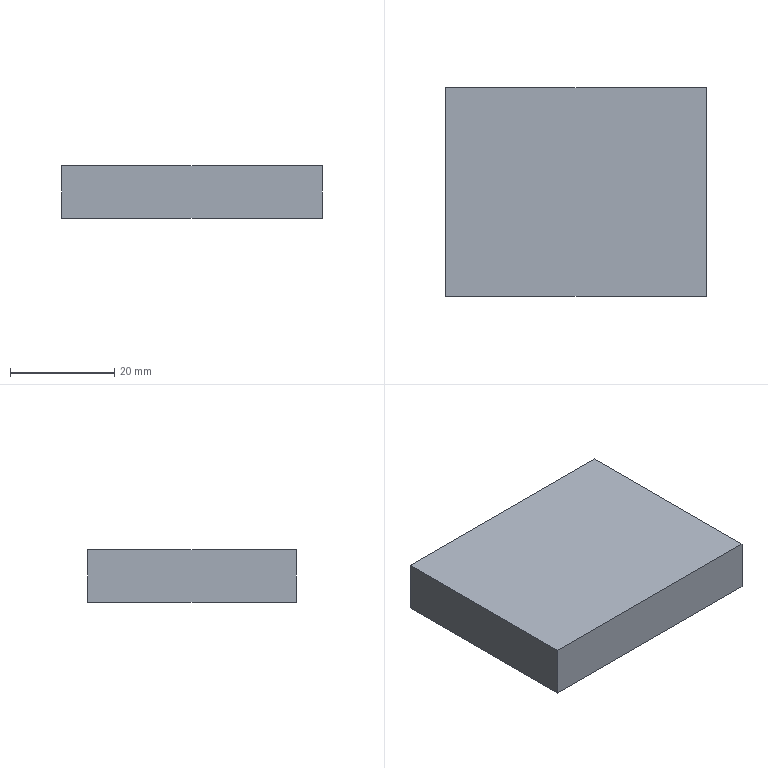Part | NX | features solid 2 | 1 solid | 6 faces | box 50 x 40 x 10 mm | volume 20000 mm3 | plane 6
STEP:
#1=CARTESIAN_POINT('',(604.,205.,-35.));
#2=VERTEX_POINT('',#1);
#3=CARTESIAN_POINT('',(604.,165.,-35.));
#4=VERTEX_POINT('',#3);
#5=CARTESIAN_POINT('',(604.,184.697,-35.));
#6=DIRECTION('',(0.,-1.,0.));
#7=VECTOR('',#6,1000.);
#8=LINE('',#5,#7);
#9=EDGE_CURVE('',#2,#4,#8,.T.);
#10=ORIENTED_EDGE('',*,*,#9,.F.);
#11=CARTESIAN_POINT('',(604.,205.,-45.));
#12=VERTEX_POINT('',#11);
#13=CARTESIAN_POINT('',(604.,205.,-45.));
#14=DIRECTION('',(0.,0.,1.));
#15=VECTOR('',#14,1000.);
#16=LINE('',#13,#15);
#17=EDGE_CURVE('',#12,#2,#16,.T.);
#18=ORIENTED_EDGE('',*,*,#17,.F.);
#19=CARTESIAN_POINT('',(604.,165.,-45.));
#20=VERTEX_POINT('',#19);
#21=CARTESIAN_POINT('',(604.,205.,-45.));
#22=DIRECTION('',(0.,1.,0.));
#23=VECTOR('',#22,1000.);
#24=LINE('',#21,#23);
#25=EDGE_CURVE('',#12,#20,#24,.F.);
#26=ORIENTED_EDGE('',*,*,#25,.T.);
#27=CARTESIAN_POINT('',(604.,165.,-50.));
#28=DIRECTION('',(0.,0.,1.));
#29=VECTOR('',#28,1000.);
#30=LINE('',#27,#29);
#31=EDGE_CURVE('',#20,#4,#30,.T.);
#32=ORIENTED_EDGE('',*,*,#31,.T.);
#33=EDGE_LOOP('',(#10,#18,#26,#32));
#34=FACE_BOUND('',#33,.T.);
#35=CARTESIAN_POINT('',(604.,205.,-45.));
#36=DIRECTION('',(1.,0.,0.));
#37=DIRECTION('',(0.,0.,-1.));
#38=AXIS2_PLACEMENT_3D('',#35,#36,#37);
#39=PLANE('',#38);
#40=ADVANCED_FACE('',(#34),#39,.F.);
#41=CARTESIAN_POINT('',(654.,205.,-35.));
#42=VERTEX_POINT('',#41);
#43=CARTESIAN_POINT('',(654.,165.,-35.));
#44=VERTEX_POINT('',#43);
#45=CARTESIAN_POINT('',(654.,184.697,-35.));
#46=DIRECTION('',(0.,1.,0.));
#47=VECTOR('',#46,1000.);
#48=LINE('',#45,#47);
#49=EDGE_CURVE('',#42,#44,#48,.F.);
#50=ORIENTED_EDGE('',*,*,#49,.T.);
#51=CARTESIAN_POINT('',(654.,165.,-45.));
#52=VERTEX_POINT('',#51);
#53=CARTESIAN_POINT('',(654.,165.,-50.));
#54=DIRECTION('',(0.,0.,-1.));
#55=VECTOR('',#54,1000.);
#56=LINE('',#53,#55);
#57=EDGE_CURVE('',#52,#44,#56,.F.);
#58=ORIENTED_EDGE('',*,*,#57,.F.);
#59=CARTESIAN_POINT('',(654.,205.,-45.));
#60=VERTEX_POINT('',#59);
#61=CARTESIAN_POINT('',(654.,205.,-45.));
#62=DIRECTION('',(0.,-1.,0.));
#63=VECTOR('',#62,1000.);
#64=LINE('',#61,#63);
#65=EDGE_CURVE('',#60,#52,#64,.T.);
#66=ORIENTED_EDGE('',*,*,#65,.F.);
#67=CARTESIAN_POINT('',(654.,205.,-55.));
#68=DIRECTION('',(0.,0.,-1.));
#69=VECTOR('',#68,1000.);
#70=LINE('',#67,#69);
#71=EDGE_CURVE('',#60,#42,#70,.F.);
#72=ORIENTED_EDGE('',*,*,#71,.T.);
#73=EDGE_LOOP('',(#50,#58,#66,#72));
#74=FACE_BOUND('',#73,.T.);
#75=CARTESIAN_POINT('',(654.,145.,-55.));
#76=DIRECTION('',(-1.,0.,0.));
#77=DIRECTION('',(0.,1.,0.));
#78=AXIS2_PLACEMENT_3D('',#75,#76,#77);
#79=PLANE('',#78);
#80=ADVANCED_FACE('',(#74),#79,.F.);
#81=ORIENTED_EDGE('',*,*,#57,.T.);
#82=CARTESIAN_POINT('',(629.,165.,-35.));
#83=DIRECTION('',(-1.,0.,0.));
#84=VECTOR('',#83,1000.);
#85=LINE('',#82,#84);
#86=EDGE_CURVE('',#44,#4,#85,.T.);
#87=ORIENTED_EDGE('',*,*,#86,.T.);
#88=ORIENTED_EDGE('',*,*,#31,.F.);
#89=CARTESIAN_POINT('',(654.,165.,-45.));
#90=DIRECTION('',(1.,0.,0.));
#91=VECTOR('',#90,1000.);
#92=LINE('',#89,#91);
#93=EDGE_CURVE('',#52,#20,#92,.F.);
#94=ORIENTED_EDGE('',*,*,#93,.F.);
#95=EDGE_LOOP('',(#81,#87,#88,#94));
#96=FACE_BOUND('',#95,.T.);
#97=CARTESIAN_POINT('',(634.,165.,-50.));
#98=DIRECTION('',(0.,-1.,0.));
#99=DIRECTION('',(-1.,0.,0.));
#100=AXIS2_PLACEMENT_3D('',#97,#98,#99);
#101=PLANE('',#100);
#102=ADVANCED_FACE('',(#96),#101,.T.);
#103=ORIENTED_EDGE('',*,*,#25,.F.);
#104=CARTESIAN_POINT('',(654.,205.,-45.));
#105=DIRECTION('',(-1.,0.,0.));
#106=VECTOR('',#105,1000.);
#107=LINE('',#104,#106);
#108=EDGE_CURVE('',#12,#60,#107,.F.);
#109=ORIENTED_EDGE('',*,*,#108,.T.);
#110=ORIENTED_EDGE('',*,*,#65,.T.);
#111=ORIENTED_EDGE('',*,*,#93,.T.);
#112=EDGE_LOOP('',(#103,#109,#110,#111));
#113=FACE_BOUND('',#112,.T.);
#114=CARTESIAN_POINT('',(654.,205.,-45.));
#115=DIRECTION('',(0.,0.,1.));
#116=DIRECTION('',(0.,-1.,0.));
#117=AXIS2_PLACEMENT_3D('',#114,#115,#116);
#118=PLANE('',#117);
#119=ADVANCED_FACE('',(#113),#118,.F.);
#120=ORIENTED_EDGE('',*,*,#108,.F.);
#121=ORIENTED_EDGE('',*,*,#17,.T.);
#122=CARTESIAN_POINT('',(629.5,205.,-35.));
#123=DIRECTION('',(-1.,0.,0.));
#124=VECTOR('',#123,1000.);
#125=LINE('',#122,#124);
#126=EDGE_CURVE('',#42,#2,#125,.T.);
#127=ORIENTED_EDGE('',*,*,#126,.F.);
#128=ORIENTED_EDGE('',*,*,#71,.F.);
#129=EDGE_LOOP('',(#120,#121,#127,#128));
#130=FACE_BOUND('',#129,.T.);
#131=CARTESIAN_POINT('',(629.5,205.,-40.721));
#132=DIRECTION('',(0.,1.,0.));
#133=DIRECTION('',(-1.,0.,0.));
#134=AXIS2_PLACEMENT_3D('',#131,#132,#133);
#135=PLANE('',#134);
#136=ADVANCED_FACE('',(#130),#135,.T.);
#137=CARTESIAN_POINT('',(644.82,181.818,-35.));
#138=VERTEX_POINT('',#137);
#139=CARTESIAN_POINT('',(613.18,181.818,-35.));
#140=VERTEX_POINT('',#139);
#141=CARTESIAN_POINT('',(629.,181.818,-35.));
#142=DIRECTION('',(-1.,0.,0.));
#143=VECTOR('',#142,1000.);
#144=LINE('',#141,#143);
#145=EDGE_CURVE('',#138,#140,#144,.T.);
#146=ORIENTED_EDGE('',*,*,#145,.F.);
#147=ORIENTED_EDGE('',*,*,#145,.T.);
#148=EDGE_LOOP('',(#146,#147));
#149=FACE_BOUND('',#148,.T.);
#150=ORIENTED_EDGE('',*,*,#86,.F.);
#151=ORIENTED_EDGE('',*,*,#49,.F.);
#152=ORIENTED_EDGE('',*,*,#126,.T.);
#153=ORIENTED_EDGE('',*,*,#9,.T.);
#154=EDGE_LOOP('',(#150,#151,#152,#153));
#155=FACE_BOUND('',#154,.T.);
#156=CARTESIAN_POINT('',(629.,184.697,-35.));
#157=DIRECTION('',(0.,0.,1.));
#158=DIRECTION('',(0.9999,0.01247,0.));
#159=AXIS2_PLACEMENT_3D('',#156,#157,#158);
#160=PLANE('',#159);
#161=ADVANCED_FACE('',(#149,#155),#160,.T.);
#162=CLOSED_SHELL('',(#40,#80,#102,#119,#136,#161));
#163=MANIFOLD_SOLID_BREP('',#162);
#164=(LENGTH_UNIT()NAMED_UNIT(*)SI_UNIT(.MILLI.,.METRE.));
#165=UNCERTAINTY_MEASURE_WITH_UNIT(LENGTH_MEASURE(0.00001),#164,'','');
#166=(NAMED_UNIT(*)PLANE_ANGLE_UNIT()SI_UNIT($,.RADIAN.));
#167=(NAMED_UNIT(*)SI_UNIT($,.STERADIAN.)SOLID_ANGLE_UNIT());
#168=(GEOMETRIC_REPRESENTATION_CONTEXT(3)GLOBAL_UNCERTAINTY_ASSIGNED_CONTEXT((#165))GLOBAL_UNIT_ASSIGNED_CONTEXT((#164,#166,#167))REPRESENTATION_CONTEXT('',''));
#169=ADVANCED_BREP_SHAPE_REPRESENTATION('',(#163),#168);